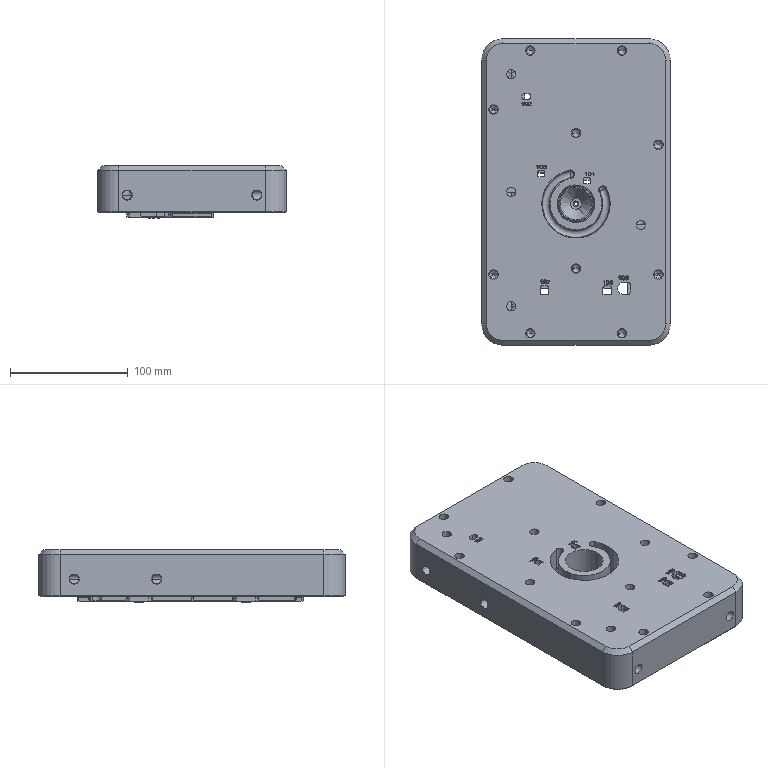Part | Creo | 1 solid | 703 faces | box 160 x 260 x 44.824 mm | volume 1550672 mm3 | plane 316 | cylinder 157 | other 132 | cone 77 | torus 15 | sphere 6 | commonest cylinder face diameters 8 x64 6.71 x20 0.402 x18 4 x8 1 x6 2.01 x4